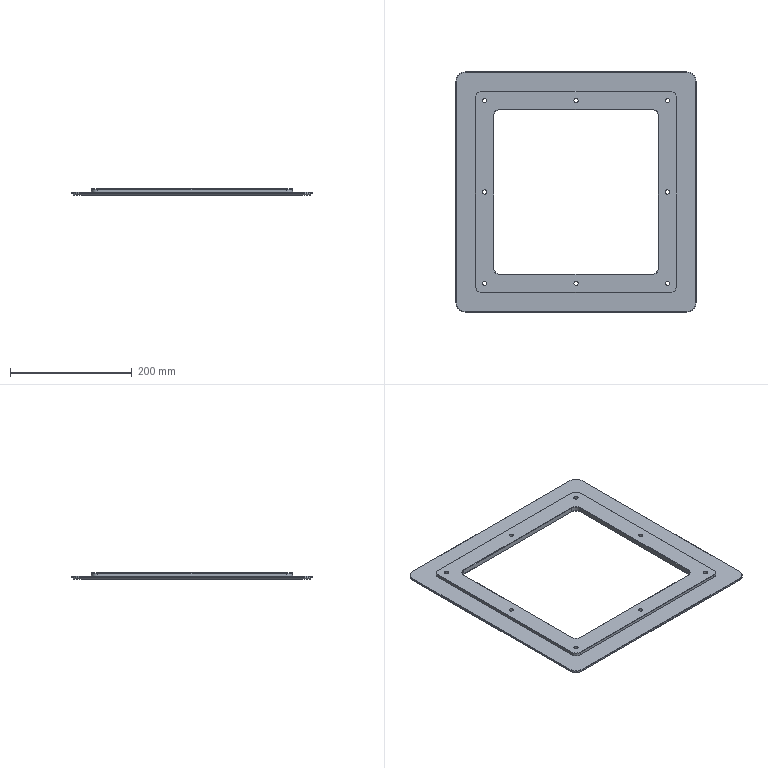Part | 1 solid | 83 faces | volume 582523 mm3 | plane 35 | cylinder 28 | cone 20 | commonest cylinder face diameters 6.8 x16 20 x8 30 x4